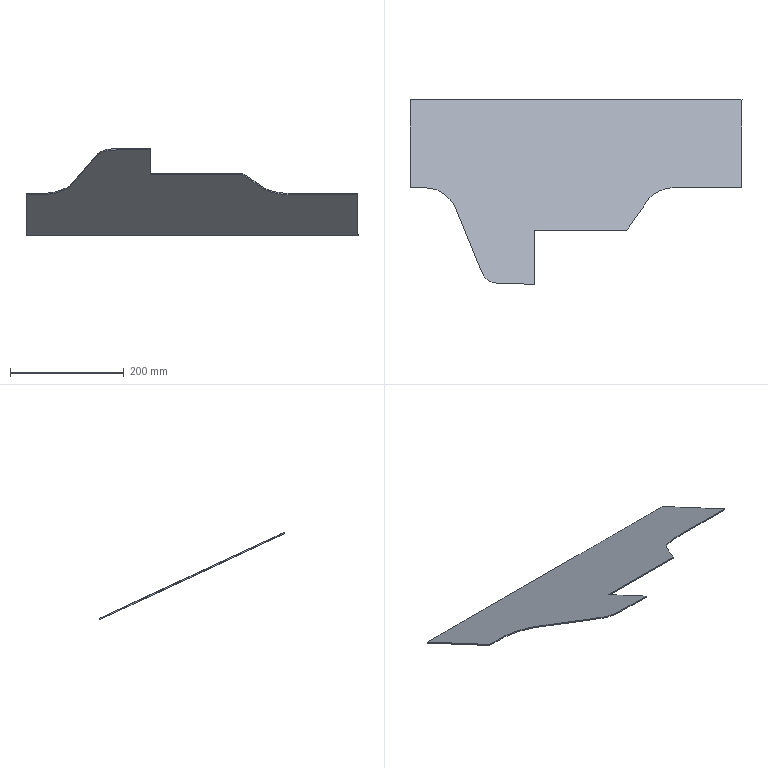Part | NX | features solid 2 | 1 solid | 9 faces | box 585 x 325.491 x 153.986 mm | volume 277101 mm3 | plane 7 | spline 2
STEP:
#1=CARTESIAN_POINT('',(-15.,64.511,-80.89));
#2=VERTEX_POINT('',#1);
#3=CARTESIAN_POINT('',(-235.,234.941,-160.363));
#4=VERTEX_POINT('',#3);
#5=CARTESIAN_POINT('',(-15.,64.511,-80.89));
#6=CARTESIAN_POINT('',(-18.445,64.501,-80.885));
#7=CARTESIAN_POINT('',(-25.333,64.55,-80.908));
#8=CARTESIAN_POINT('',(-35.665,64.778,-81.014));
#9=CARTESIAN_POINT('',(-45.997,65.047,-81.14));
#10=CARTESIAN_POINT('',(-56.325,65.488,-81.346));
#11=CARTESIAN_POINT('',(-66.665,65.754,-81.47));
#12=CARTESIAN_POINT('',(-76.969,65.677,-81.434));
#13=CARTESIAN_POINT('',(-87.409,66.786,-81.951));
#14=CARTESIAN_POINT('',(-97.044,70.795,-83.82));
#15=CARTESIAN_POINT('',(-104.46,77.651,-87.017));
#16=CARTESIAN_POINT('',(-109.205,86.072,-90.944));
#17=CARTESIAN_POINT('',(-112.555,95.072,-95.141));
#18=CARTESIAN_POINT('',(-115.959,104.022,-99.314));
#19=CARTESIAN_POINT('',(-119.506,112.932,-103.469));
#20=CARTESIAN_POINT('',(-123.05,121.84,-107.623));
#21=CARTESIAN_POINT('',(-126.716,130.709,-111.759));
#22=CARTESIAN_POINT('',(-131.727,142.492,-117.253));
#23=CARTESIAN_POINT('',(-138.057,157.199,-124.111));
#24=CARTESIAN_POINT('',(-144.248,171.953,-130.991));
#25=CARTESIAN_POINT('',(-148.845,183.875,-136.55));
#26=CARTESIAN_POINT('',(-152.222,192.846,-140.733));
#27=CARTESIAN_POINT('',(-155.816,201.72,-144.872));
#28=CARTESIAN_POINT('',(-160.656,210.149,-148.802));
#29=CARTESIAN_POINT('',(-167.167,217.758,-152.35));
#30=CARTESIAN_POINT('',(-174.848,224.259,-155.382));
#31=CARTESIAN_POINT('',(-183.675,229.58,-157.863));
#32=CARTESIAN_POINT('',(-191.706,232.657,-159.298));
#33=CARTESIAN_POINT('',(-198.651,234.08,-159.962));
#34=CARTESIAN_POINT('',(-205.542,234.889,-160.338));
#35=CARTESIAN_POINT('',(-214.207,235.059,-160.418));
#36=CARTESIAN_POINT('',(-224.604,234.94,-160.362));
#37=CARTESIAN_POINT('',(-231.535,234.942,-160.363));
#38=CARTESIAN_POINT('',(-235.,234.941,-160.363));
#39=B_SPLINE_CURVE_WITH_KNOTS('',3,(#5,#6,#7,#8,#9,#10,#11,#12,#13,#14,#15,#16,#17,#18,#19,#20,#21,#22,#23,#24,#25,#26,#27,#28,#29,#30,#31,#32,#33,#34,#35,#36,#37,#38),.UNSPECIFIED.,.F.,.F.,(4,1,1,1,1,1,1,1,1,1,1,1,1,1,1,1,1,1,1,1,1,1,1,1,1,1,1,1,1,1,1,4),(0.4481,0.4583,0.4685,0.4788,0.489,0.4992,0.5095,0.5197,0.5299,0.5402,0.5504,0.5606,0.5709,0.5811,0.5914,0.6016,0.6118,0.6323,0.6528,0.663,0.6732,0.6835,0.6937,0.7039,0.7142,0.7244,0.7346,0.7398,0.7449,0.7551,0.7654,0.7756),.UNSPECIFIED.);
#40=EDGE_CURVE('',#2,#4,#39,.T.);
#41=ORIENTED_EDGE('',*,*,#40,.F.);
#42=CARTESIAN_POINT('',(-15.,160.,-125.417));
#43=VERTEX_POINT('',#42);
#44=CARTESIAN_POINT('',(-15.,512.511,-289.796));
#45=DIRECTION('',(0.,0.9063,-0.4226));
#46=VECTOR('',#45,1000.);
#47=LINE('',#44,#46);
#48=EDGE_CURVE('',#2,#43,#47,.T.);
#49=ORIENTED_EDGE('',*,*,#48,.T.);
#50=CARTESIAN_POINT('',(147.311,160.,-125.417));
#51=VERTEX_POINT('',#50);
#52=CARTESIAN_POINT('',(45.,160.,-125.417));
#53=DIRECTION('',(1.,0.,0.));
#54=VECTOR('',#53,1000.);
#55=LINE('',#52,#54);
#56=EDGE_CURVE('',#43,#51,#55,.T.);
#57=ORIENTED_EDGE('',*,*,#56,.T.);
#58=CARTESIAN_POINT('',(350.,234.942,-160.363));
#59=VERTEX_POINT('',#58);
#60=CARTESIAN_POINT('',(350.,234.942,-160.363));
#61=CARTESIAN_POINT('',(339.975,234.936,-160.361));
#62=CARTESIAN_POINT('',(324.937,234.935,-160.36));
#63=CARTESIAN_POINT('',(304.886,234.96,-160.372));
#64=CARTESIAN_POINT('',(289.848,234.985,-160.383));
#65=CARTESIAN_POINT('',(274.811,234.996,-160.388));
#66=CARTESIAN_POINT('',(259.772,234.948,-160.366));
#67=CARTESIAN_POINT('',(247.244,234.881,-160.335));
#68=CARTESIAN_POINT('',(237.205,235.037,-160.408));
#69=CARTESIAN_POINT('',(229.686,235.041,-160.41));
#70=CARTESIAN_POINT('',(222.219,234.482,-160.149));
#71=CARTESIAN_POINT('',(214.845,233.031,-159.472));
#72=CARTESIAN_POINT('',(207.533,230.61,-158.343));
#73=CARTESIAN_POINT('',(200.799,227.39,-156.842));
#74=CARTESIAN_POINT('',(194.539,223.399,-154.981));
#75=CARTESIAN_POINT('',(188.818,218.647,-152.765));
#76=CARTESIAN_POINT('',(183.898,213.367,-150.303));
#77=CARTESIAN_POINT('',(179.607,207.587,-147.608));
#78=CARTESIAN_POINT('',(175.69,201.565,-144.799));
#79=CARTESIAN_POINT('',(170.518,193.522,-141.049));
#80=CARTESIAN_POINT('',(163.791,183.604,-136.424));
#81=CARTESIAN_POINT('',(155.579,171.787,-130.914));
#82=CARTESIAN_POINT('',(150.08,163.921,-127.246));
#83=CARTESIAN_POINT('',(147.311,160.,-125.417));
#84=B_SPLINE_CURVE_WITH_KNOTS('',3,(#60,#61,#62,#63,#64,#65,#66,#67,#68,#69,#70,#71,#72,#73,#74,#75,#76,#77,#78,#79,#80,#81,#82,#83),.UNSPECIFIED.,.F.,.F.,(4,1,1,1,1,1,1,1,1,1,1,1,1,1,1,1,1,1,1,1,1,4),(0.,0.03008,0.04511,0.06015,0.07519,0.09023,0.1053,0.1128,0.1203,0.1278,0.1353,0.1429,0.1504,0.1579,0.1654,0.1729,0.1805,0.188,0.1955,0.2105,0.2256,0.2406),.UNSPECIFIED.);
#85=EDGE_CURVE('',#59,#51,#84,.T.);
#86=ORIENTED_EDGE('',*,*,#85,.F.);
#87=CARTESIAN_POINT('',(350.,390.,-232.668));
#88=VERTEX_POINT('',#87);
#89=CARTESIAN_POINT('',(350.,287.2,-184.732));
#90=DIRECTION('',(0.,-0.9063,0.4226));
#91=VECTOR('',#90,1000.);
#92=LINE('',#89,#91);
#93=EDGE_CURVE('',#88,#59,#92,.T.);
#94=ORIENTED_EDGE('',*,*,#93,.F.);
#95=CARTESIAN_POINT('',(-235.,390.,-232.668));
#96=VERTEX_POINT('',#95);
#97=CARTESIAN_POINT('',(45.,390.,-232.668));
#98=DIRECTION('',(-1.,0.,0.));
#99=VECTOR('',#98,1000.);
#100=LINE('',#97,#99);
#101=EDGE_CURVE('',#88,#96,#100,.T.);
#102=ORIENTED_EDGE('',*,*,#101,.T.);
#103=CARTESIAN_POINT('',(-235.,512.511,-289.796));
#104=DIRECTION('',(0.,0.9063,-0.4226));
#105=VECTOR('',#104,1000.);
#106=LINE('',#103,#105);
#107=EDGE_CURVE('',#96,#4,#106,.F.);
#108=ORIENTED_EDGE('',*,*,#107,.T.);
#109=EDGE_LOOP('',(#41,#49,#57,#86,#94,#102,#108));
#110=FACE_BOUND('',#109,.T.);
#111=CARTESIAN_POINT('',(45.,512.511,-289.796));
#112=DIRECTION('',(0.,0.4226,0.9063));
#113=DIRECTION('',(1.,0.,0.));
#114=AXIS2_PLACEMENT_3D('',#111,#112,#113);
#115=PLANE('',#114);
#116=ADVANCED_FACE('',(#110),#115,.T.);
#117=CARTESIAN_POINT('',(-15.,64.511,-83.097));
#118=VERTEX_POINT('',#117);
#119=CARTESIAN_POINT('',(-15.,160.,-127.624));
#120=VERTEX_POINT('',#119);
#121=CARTESIAN_POINT('',(-15.,175.818,-135.));
#122=DIRECTION('',(0.,0.9063,-0.4226));
#123=VECTOR('',#122,1000.);
#124=LINE('',#121,#123);
#125=EDGE_CURVE('',#118,#120,#124,.T.);
#126=ORIENTED_EDGE('',*,*,#125,.F.);
#127=CARTESIAN_POINT('',(-235.,234.941,-162.57));
#128=VERTEX_POINT('',#127);
#129=CARTESIAN_POINT('',(-15.,64.511,-83.097));
#130=CARTESIAN_POINT('',(-18.445,64.501,-83.092));
#131=CARTESIAN_POINT('',(-25.333,64.55,-83.115));
#132=CARTESIAN_POINT('',(-35.665,64.778,-83.221));
#133=CARTESIAN_POINT('',(-45.997,65.047,-83.347));
#134=CARTESIAN_POINT('',(-56.325,65.488,-83.552));
#135=CARTESIAN_POINT('',(-66.665,65.754,-83.676));
#136=CARTESIAN_POINT('',(-76.969,65.677,-83.641));
#137=CARTESIAN_POINT('',(-87.409,66.786,-84.158));
#138=CARTESIAN_POINT('',(-97.044,70.795,-86.027));
#139=CARTESIAN_POINT('',(-104.46,77.651,-89.224));
#140=CARTESIAN_POINT('',(-109.205,86.072,-93.151));
#141=CARTESIAN_POINT('',(-112.555,95.072,-97.348));
#142=CARTESIAN_POINT('',(-115.959,104.022,-101.521));
#143=CARTESIAN_POINT('',(-119.506,112.932,-105.676));
#144=CARTESIAN_POINT('',(-123.05,121.84,-109.83));
#145=CARTESIAN_POINT('',(-126.716,130.709,-113.965));
#146=CARTESIAN_POINT('',(-131.727,142.492,-119.46));
#147=CARTESIAN_POINT('',(-138.057,157.199,-126.318));
#148=CARTESIAN_POINT('',(-144.248,171.953,-133.198));
#149=CARTESIAN_POINT('',(-148.845,183.875,-138.757));
#150=CARTESIAN_POINT('',(-152.222,192.846,-142.94));
#151=CARTESIAN_POINT('',(-155.816,201.72,-147.078));
#152=CARTESIAN_POINT('',(-160.656,210.149,-151.009));
#153=CARTESIAN_POINT('',(-167.167,217.758,-154.557));
#154=CARTESIAN_POINT('',(-174.848,224.259,-157.588));
#155=CARTESIAN_POINT('',(-183.675,229.58,-160.07));
#156=CARTESIAN_POINT('',(-191.706,232.657,-161.504));
#157=CARTESIAN_POINT('',(-198.651,234.08,-162.168));
#158=CARTESIAN_POINT('',(-205.542,234.889,-162.545));
#159=CARTESIAN_POINT('',(-214.207,235.059,-162.624));
#160=CARTESIAN_POINT('',(-224.604,234.94,-162.569));
#161=CARTESIAN_POINT('',(-231.535,234.942,-162.57));
#162=CARTESIAN_POINT('',(-235.,234.941,-162.57));
#163=B_SPLINE_CURVE_WITH_KNOTS('',3,(#129,#130,#131,#132,#133,#134,#135,#136,#137,#138,#139,#140,#141,#142,#143,#144,#145,#146,#147,#148,#149,#150,#151,#152,#153,#154,#155,#156,#157,#158,#159,#160,#161,#162),.UNSPECIFIED.,.F.,.F.,(4,1,1,1,1,1,1,1,1,1,1,1,1,1,1,1,1,1,1,1,1,1,1,1,1,1,1,1,1,1,1,4),(0.4481,0.4583,0.4685,0.4788,0.489,0.4992,0.5095,0.5197,0.5299,0.5402,0.5504,0.5606,0.5709,0.5811,0.5914,0.6016,0.6118,0.6323,0.6528,0.663,0.6732,0.6835,0.6937,0.7039,0.7142,0.7244,0.7346,0.7398,0.7449,0.7551,0.7654,0.7756),.UNSPECIFIED.);
#164=EDGE_CURVE('',#118,#128,#163,.T.);
#165=ORIENTED_EDGE('',*,*,#164,.T.);
#166=CARTESIAN_POINT('',(-235.,390.,-234.875));
#167=VERTEX_POINT('',#166);
#168=CARTESIAN_POINT('',(-235.,175.818,-135.));
#169=DIRECTION('',(0.,0.9063,-0.4226));
#170=VECTOR('',#169,1000.);
#171=LINE('',#168,#170);
#172=EDGE_CURVE('',#167,#128,#171,.F.);
#173=ORIENTED_EDGE('',*,*,#172,.F.);
#174=CARTESIAN_POINT('',(350.,390.,-234.875));
#175=VERTEX_POINT('',#174);
#176=CARTESIAN_POINT('',(-950.,390.,-234.875));
#177=DIRECTION('',(-1.,0.,0.));
#178=VECTOR('',#177,1000.);
#179=LINE('',#176,#178);
#180=EDGE_CURVE('',#175,#167,#179,.T.);
#181=ORIENTED_EDGE('',*,*,#180,.F.);
#182=CARTESIAN_POINT('',(350.,234.942,-162.57));
#183=VERTEX_POINT('',#182);
#184=CARTESIAN_POINT('',(350.,286.355,-186.544));
#185=DIRECTION('',(0.,-0.9063,0.4226));
#186=VECTOR('',#185,1000.);
#187=LINE('',#184,#186);
#188=EDGE_CURVE('',#175,#183,#187,.T.);
#189=ORIENTED_EDGE('',*,*,#188,.T.);
#190=CARTESIAN_POINT('',(147.311,160.,-127.624));
#191=VERTEX_POINT('',#190);
#192=CARTESIAN_POINT('',(350.,234.942,-162.57));
#193=CARTESIAN_POINT('',(339.975,234.936,-162.567));
#194=CARTESIAN_POINT('',(324.937,234.935,-162.567));
#195=CARTESIAN_POINT('',(304.886,234.96,-162.579));
#196=CARTESIAN_POINT('',(289.848,234.985,-162.59));
#197=CARTESIAN_POINT('',(274.811,234.996,-162.595));
#198=CARTESIAN_POINT('',(259.772,234.948,-162.573));
#199=CARTESIAN_POINT('',(247.244,234.881,-162.542));
#200=CARTESIAN_POINT('',(237.205,235.037,-162.614));
#201=CARTESIAN_POINT('',(229.686,235.041,-162.616));
#202=CARTESIAN_POINT('',(222.219,234.482,-162.356));
#203=CARTESIAN_POINT('',(214.845,233.031,-161.679));
#204=CARTESIAN_POINT('',(207.533,230.61,-160.55));
#205=CARTESIAN_POINT('',(200.799,227.39,-159.048));
#206=CARTESIAN_POINT('',(194.539,223.399,-157.187));
#207=CARTESIAN_POINT('',(188.818,218.647,-154.972));
#208=CARTESIAN_POINT('',(183.898,213.367,-152.509));
#209=CARTESIAN_POINT('',(179.607,207.587,-149.814));
#210=CARTESIAN_POINT('',(175.69,201.565,-147.006));
#211=CARTESIAN_POINT('',(170.518,193.522,-143.255));
#212=CARTESIAN_POINT('',(163.791,183.604,-138.631));
#213=CARTESIAN_POINT('',(155.579,171.787,-133.12));
#214=CARTESIAN_POINT('',(150.08,163.921,-129.453));
#215=CARTESIAN_POINT('',(147.311,160.,-127.624));
#216=B_SPLINE_CURVE_WITH_KNOTS('',3,(#192,#193,#194,#195,#196,#197,#198,#199,#200,#201,#202,#203,#204,#205,#206,#207,#208,#209,#210,#211,#212,#213,#214,#215),.UNSPECIFIED.,.F.,.F.,(4,1,1,1,1,1,1,1,1,1,1,1,1,1,1,1,1,1,1,1,1,4),(0.,0.03008,0.04511,0.06015,0.07519,0.09023,0.1053,0.1128,0.1203,0.1278,0.1353,0.1429,0.1504,0.1579,0.1654,0.1729,0.1805,0.188,0.1955,0.2105,0.2256,0.2406),.UNSPECIFIED.);
#217=EDGE_CURVE('',#183,#191,#216,.T.);
#218=ORIENTED_EDGE('',*,*,#217,.T.);
#219=CARTESIAN_POINT('',(-950.,160.,-127.624));
#220=DIRECTION('',(1.,0.,0.));
#221=VECTOR('',#220,1000.);
#222=LINE('',#219,#221);
#223=EDGE_CURVE('',#120,#191,#222,.T.);
#224=ORIENTED_EDGE('',*,*,#223,.F.);
#225=EDGE_LOOP('',(#126,#165,#173,#181,#189,#218,#224));
#226=FACE_BOUND('',#225,.T.);
#227=CARTESIAN_POINT('',(-950.,175.818,-135.));
#228=DIRECTION('',(0.,0.4226,0.9063));
#229=DIRECTION('',(0.,-0.9063,0.4226));
#230=AXIS2_PLACEMENT_3D('',#227,#228,#229);
#231=PLANE('',#230);
#232=ADVANCED_FACE('',(#226),#231,.F.);
#233=ORIENTED_EDGE('',*,*,#101,.F.);
#234=CARTESIAN_POINT('',(350.,390.,-145.));
#235=DIRECTION('',(0.,0.,-1.));
#236=VECTOR('',#235,1000.);
#237=LINE('',#234,#236);
#238=EDGE_CURVE('',#88,#175,#237,.T.);
#239=ORIENTED_EDGE('',*,*,#238,.T.);
#240=ORIENTED_EDGE('',*,*,#180,.T.);
#241=CARTESIAN_POINT('',(-235.,390.,-327.54));
#242=DIRECTION('',(0.,0.,1.));
#243=VECTOR('',#242,1000.);
#244=LINE('',#241,#243);
#245=EDGE_CURVE('',#96,#167,#244,.F.);
#246=ORIENTED_EDGE('',*,*,#245,.F.);
#247=EDGE_LOOP('',(#233,#239,#240,#246));
#248=FACE_BOUND('',#247,.T.);
#249=CARTESIAN_POINT('',(455.,390.,-145.));
#250=DIRECTION('',(0.,1.,0.));
#251=DIRECTION('',(0.,0.,-1.));
#252=AXIS2_PLACEMENT_3D('',#249,#250,#251);
#253=PLANE('',#252);
#254=ADVANCED_FACE('',(#248),#253,.T.);
#255=CARTESIAN_POINT('',(-15.,64.511,-121.239));
#256=DIRECTION('',(0.,0.,-1.));
#257=VECTOR('',#256,1000.);
#258=LINE('',#255,#257);
#259=EDGE_CURVE('',#2,#118,#258,.T.);
#260=ORIENTED_EDGE('',*,*,#259,.F.);
#261=ORIENTED_EDGE('',*,*,#40,.T.);
#262=CARTESIAN_POINT('',(-235.,234.941,-161.472));
#263=DIRECTION('',(0.,0.,-1.));
#264=VECTOR('',#263,1000.);
#265=LINE('',#262,#264);
#266=EDGE_CURVE('',#4,#128,#265,.T.);
#267=ORIENTED_EDGE('',*,*,#266,.T.);
#268=ORIENTED_EDGE('',*,*,#164,.F.);
#269=EDGE_LOOP('',(#260,#261,#267,#268));
#270=FACE_BOUND('',#269,.T.);
#271=CARTESIAN_POINT('',(-235.,234.941,-79.524));
#272=CARTESIAN_POINT('',(-235.,234.941,-163.701));
#273=CARTESIAN_POINT('',(-231.678,234.942,-79.524));
#274=CARTESIAN_POINT('',(-231.678,234.942,-163.701));
#275=CARTESIAN_POINT('',(-225.038,234.941,-79.524));
#276=CARTESIAN_POINT('',(-225.038,234.941,-163.701));
#277=CARTESIAN_POINT('',(-215.058,235.044,-79.524));
#278=CARTESIAN_POINT('',(-215.058,235.044,-163.701));
#279=CARTESIAN_POINT('',(-205.091,234.915,-79.524));
#280=CARTESIAN_POINT('',(-205.091,234.915,-163.701));
#281=CARTESIAN_POINT('',(-195.172,233.672,-79.524));
#282=CARTESIAN_POINT('',(-195.172,233.672,-163.701));
#283=CARTESIAN_POINT('',(-185.67,230.508,-79.524));
#284=CARTESIAN_POINT('',(-185.67,230.508,-163.701));
#285=CARTESIAN_POINT('',(-176.916,225.67,-79.524));
#286=CARTESIAN_POINT('',(-176.916,225.67,-163.701));
#287=CARTESIAN_POINT('',(-169.03,219.526,-79.524));
#288=CARTESIAN_POINT('',(-169.03,219.526,-163.701));
#289=CARTESIAN_POINT('',(-162.191,212.204,-79.524));
#290=CARTESIAN_POINT('',(-162.191,212.204,-163.701));
#291=CARTESIAN_POINT('',(-156.804,203.807,-79.524));
#292=CARTESIAN_POINT('',(-156.804,203.807,-163.701));
#293=CARTESIAN_POINT('',(-152.887,194.628,-79.524));
#294=CARTESIAN_POINT('',(-152.887,194.628,-163.701));
#295=CARTESIAN_POINT('',(-149.376,185.265,-79.524));
#296=CARTESIAN_POINT('',(-149.376,185.265,-163.701));
#297=CARTESIAN_POINT('',(-144.62,172.874,-79.524));
#298=CARTESIAN_POINT('',(-144.62,172.874,-163.701));
#299=CARTESIAN_POINT('',(-138.21,157.543,-79.524));
#300=CARTESIAN_POINT('',(-138.21,157.543,-163.701));
#301=CARTESIAN_POINT('',(-131.638,142.287,-79.524));
#302=CARTESIAN_POINT('',(-131.638,142.287,-163.701));
#303=CARTESIAN_POINT('',(-126.44,130.056,-79.524));
#304=CARTESIAN_POINT('',(-126.44,130.056,-163.701));
#305=CARTESIAN_POINT('',(-122.644,120.84,-79.524));
#306=CARTESIAN_POINT('',(-122.644,120.84,-163.701));
#307=CARTESIAN_POINT('',(-118.971,111.575,-79.524));
#308=CARTESIAN_POINT('',(-118.971,111.575,-163.701));
#309=CARTESIAN_POINT('',(-115.278,102.315,-79.524));
#310=CARTESIAN_POINT('',(-115.278,102.315,-163.701));
#311=CARTESIAN_POINT('',(-111.803,92.98,-79.524));
#312=CARTESIAN_POINT('',(-111.803,92.98,-163.701));
#313=CARTESIAN_POINT('',(-108.16,83.678,-79.524));
#314=CARTESIAN_POINT('',(-108.16,83.678,-163.701));
#315=CARTESIAN_POINT('',(-102.524,75.335,-79.524));
#316=CARTESIAN_POINT('',(-102.524,75.335,-163.701));
#317=CARTESIAN_POINT('',(-94.368,69.314,-79.524));
#318=CARTESIAN_POINT('',(-94.368,69.314,-163.701));
#319=CARTESIAN_POINT('',(-84.772,66.318,-79.524));
#320=CARTESIAN_POINT('',(-84.772,66.318,-163.701));
#321=CARTESIAN_POINT('',(-74.812,65.672,-79.524));
#322=CARTESIAN_POINT('',(-74.812,65.672,-163.701));
#323=CARTESIAN_POINT('',(-64.802,65.749,-79.524));
#324=CARTESIAN_POINT('',(-64.802,65.749,-163.701));
#325=CARTESIAN_POINT('',(-54.86,65.409,-79.524));
#326=CARTESIAN_POINT('',(-54.86,65.409,-163.701));
#327=CARTESIAN_POINT('',(-44.895,65.018,-79.524));
#328=CARTESIAN_POINT('',(-44.895,65.018,-163.701));
#329=CARTESIAN_POINT('',(-31.612,64.671,-79.524));
#330=CARTESIAN_POINT('',(-31.612,64.671,-163.701));
#331=CARTESIAN_POINT('',(-21.645,64.492,-79.524));
#332=CARTESIAN_POINT('',(-21.645,64.492,-163.701));
#333=CARTESIAN_POINT('',(-15.,64.511,-79.524));
#334=CARTESIAN_POINT('',(-15.,64.511,-163.701));
#335=B_SPLINE_SURFACE_WITH_KNOTS('',3,1,((#271,#272),(#273,#274),(#275,#276),(#277,#278),(#279,#280),(#281,#282),(#283,#284),(#285,#286),(#287,#288),(#289,#290),(#291,#292),(#293,#294),(#295,#296),(#297,#298),(#299,#300),(#301,#302),(#303,#304),(#305,#306),(#307,#308),(#309,#310),(#311,#312),(#313,#314),(#315,#316),(#317,#318),(#319,#320),(#321,#322),(#323,#324),(#325,#326),(#327,#328),(#329,#330),(#331,#332),(#333,#334)),.SURF_OF_LINEAR_EXTRUSION.,.F.,.F.,.F.,(4,1,1,1,1,1,1,1,1,1,1,1,1,1,1,1,1,1,1,1,1,1,1,1,1,1,1,1,1,4),(2,2),(0.6464,0.6486,0.6508,0.653,0.6552,0.6574,0.6596,0.6618,0.6639,0.6661,0.6683,0.6705,0.6727,0.6771,0.6815,0.6837,0.6859,0.6881,0.6903,0.6924,0.6946,0.6968,0.699,0.7012,0.7034,0.7056,0.7078,0.71,0.7122,0.7166),(0.,1.),.UNSPECIFIED.);
#336=ADVANCED_FACE('',(#270),#335,.F.);
#337=ORIENTED_EDGE('',*,*,#266,.F.);
#338=ORIENTED_EDGE('',*,*,#107,.F.);
#339=ORIENTED_EDGE('',*,*,#245,.T.);
#340=ORIENTED_EDGE('',*,*,#172,.T.);
#341=EDGE_LOOP('',(#337,#338,#339,#340));
#342=FACE_BOUND('',#341,.T.);
#343=CARTESIAN_POINT('',(-235.,154.934,-327.54));
#344=DIRECTION('',(1.,-0.000000001,0.));
#345=DIRECTION('',(0.000000001,1.,0.));
#346=AXIS2_PLACEMENT_3D('',#343,#344,#345);
#347=PLANE('',#346);
#348=ADVANCED_FACE('',(#342),#347,.F.);
#349=CARTESIAN_POINT('',(-15.,160.,-415.));
#350=DIRECTION('',(0.,0.,-1.));
#351=VECTOR('',#350,1000.);
#352=LINE('',#349,#351);
#353=EDGE_CURVE('',#43,#120,#352,.T.);
#354=ORIENTED_EDGE('',*,*,#353,.F.);
#355=ORIENTED_EDGE('',*,*,#48,.F.);
#356=ORIENTED_EDGE('',*,*,#259,.T.);
#357=ORIENTED_EDGE('',*,*,#125,.T.);
#358=EDGE_LOOP('',(#354,#355,#356,#357));
#359=FACE_BOUND('',#358,.T.);
#360=CARTESIAN_POINT('',(-15.,160.,-415.));
#361=DIRECTION('',(1.,0.,0.));
#362=DIRECTION('',(0.,0.,-1.));
#363=AXIS2_PLACEMENT_3D('',#360,#361,#362);
#364=PLANE('',#363);
#365=ADVANCED_FACE('',(#359),#364,.T.);
#366=CARTESIAN_POINT('',(147.311,160.,-121.582));
#367=DIRECTION('',(0.,0.,-1.));
#368=VECTOR('',#367,1000.);
#369=LINE('',#366,#368);
#370=EDGE_CURVE('',#191,#51,#369,.F.);
#371=ORIENTED_EDGE('',*,*,#370,.F.);
#372=ORIENTED_EDGE('',*,*,#217,.F.);
#373=CARTESIAN_POINT('',(350.,234.942,600.));
#374=DIRECTION('',(0.,0.,-1.));
#375=VECTOR('',#374,1000.);
#376=LINE('',#373,#375);
#377=EDGE_CURVE('',#183,#59,#376,.F.);
#378=ORIENTED_EDGE('',*,*,#377,.T.);
#379=ORIENTED_EDGE('',*,*,#85,.T.);
#380=EDGE_LOOP('',(#371,#372,#378,#379));
#381=FACE_BOUND('',#380,.T.);
#382=CARTESIAN_POINT('',(147.311,160.,-125.192));
#383=CARTESIAN_POINT('',(147.311,160.,-163.23));
#384=CARTESIAN_POINT('',(150.161,164.036,-125.192));
#385=CARTESIAN_POINT('',(150.161,164.036,-163.23));
#386=CARTESIAN_POINT('',(155.821,172.137,-125.192));
#387=CARTESIAN_POINT('',(155.821,172.137,-163.23));
#388=CARTESIAN_POINT('',(164.284,184.309,-125.192));
#389=CARTESIAN_POINT('',(164.284,184.309,-163.23));
#390=CARTESIAN_POINT('',(171.195,194.546,-125.192));
#391=CARTESIAN_POINT('',(171.195,194.546,-163.23));
#392=CARTESIAN_POINT('',(176.52,202.872,-125.192));
#393=CARTESIAN_POINT('',(176.52,202.872,-163.23));
#394=CARTESIAN_POINT('',(180.617,209.051,-125.192));
#395=CARTESIAN_POINT('',(180.617,209.051,-163.23));
#396=CARTESIAN_POINT('',(185.186,214.9,-125.192));
#397=CARTESIAN_POINT('',(185.186,214.9,-163.23));
#398=CARTESIAN_POINT('',(192.209,221.88,-125.192));
#399=CARTESIAN_POINT('',(192.209,221.88,-163.23));
#400=CARTESIAN_POINT('',(202.539,228.833,-125.192));
#401=CARTESIAN_POINT('',(202.539,228.833,-163.23));
#402=CARTESIAN_POINT('',(214.238,233.067,-125.192));
#403=CARTESIAN_POINT('',(214.238,233.067,-163.23));
#404=CARTESIAN_POINT('',(224.006,234.693,-125.192));
#405=CARTESIAN_POINT('',(224.006,234.693,-163.23));
#406=CARTESIAN_POINT('',(231.403,235.07,-125.192));
#407=CARTESIAN_POINT('',(231.403,235.07,-163.23));
#408=CARTESIAN_POINT('',(238.823,235.006,-125.192));
#409=CARTESIAN_POINT('',(238.823,235.006,-163.23));
#410=CARTESIAN_POINT('',(248.712,234.881,-125.192));
#411=CARTESIAN_POINT('',(248.712,234.881,-163.23));
#412=CARTESIAN_POINT('',(261.058,234.957,-125.192));
#413=CARTESIAN_POINT('',(261.058,234.957,-163.23));
#414=CARTESIAN_POINT('',(275.883,234.996,-125.192));
#415=CARTESIAN_POINT('',(275.883,234.996,-163.23));
#416=CARTESIAN_POINT('',(290.707,234.984,-125.192));
#417=CARTESIAN_POINT('',(290.707,234.984,-163.23));
#418=CARTESIAN_POINT('',(305.53,234.959,-125.192));
#419=CARTESIAN_POINT('',(305.53,234.959,-163.23));
#420=CARTESIAN_POINT('',(325.294,234.935,-125.192));
#421=CARTESIAN_POINT('',(325.294,234.935,-163.23));
#422=CARTESIAN_POINT('',(340.118,234.936,-125.192));
#423=CARTESIAN_POINT('',(340.118,234.936,-163.23));
#424=CARTESIAN_POINT('',(350.,234.942,-125.192));
#425=CARTESIAN_POINT('',(350.,234.942,-163.23));
#426=B_SPLINE_SURFACE_WITH_KNOTS('',3,1,((#382,#383),(#384,#385),(#386,#387),(#388,#389),(#390,#391),(#392,#393),(#394,#395),(#396,#397),(#398,#399),(#400,#401),(#402,#403),(#404,#405),(#406,#407),(#408,#409),(#410,#411),(#412,#413),(#414,#415),(#416,#417),(#418,#419),(#420,#421),(#422,#423),(#424,#425)),.SURF_OF_LINEAR_EXTRUSION.,.F.,.F.,.F.,(4,1,1,1,1,1,1,1,1,1,1,1,1,1,1,1,1,1,1,4),(2,2),(0.7617,0.7649,0.7682,0.7715,0.7731,0.7747,0.7763,0.778,0.7812,0.7845,0.7861,0.7878,0.7894,0.791,0.7943,0.7975,0.8008,0.8041,0.8073,0.8138),(0.,1.),.UNSPECIFIED.);
#427=ADVANCED_FACE('',(#381),#426,.F.);
#428=ORIENTED_EDGE('',*,*,#377,.F.);
#429=ORIENTED_EDGE('',*,*,#188,.F.);
#430=ORIENTED_EDGE('',*,*,#238,.F.);
#431=ORIENTED_EDGE('',*,*,#93,.T.);
#432=EDGE_LOOP('',(#428,#429,#430,#431));
#433=FACE_BOUND('',#432,.T.);
#434=CARTESIAN_POINT('',(350.,229.934,-307.54));
#435=DIRECTION('',(1.,0.,0.));
#436=DIRECTION('',(0.,1.,0.));
#437=AXIS2_PLACEMENT_3D('',#434,#435,#436);
#438=PLANE('',#437);
#439=ADVANCED_FACE('',(#433),#438,.T.);
#440=ORIENTED_EDGE('',*,*,#223,.T.);
#441=ORIENTED_EDGE('',*,*,#370,.T.);
#442=ORIENTED_EDGE('',*,*,#56,.F.);
#443=ORIENTED_EDGE('',*,*,#353,.T.);
#444=EDGE_LOOP('',(#440,#441,#442,#443));
#445=FACE_BOUND('',#444,.T.);
#446=CARTESIAN_POINT('',(5.,160.,-125.));
#447=DIRECTION('',(0.,-1.,0.));
#448=DIRECTION('',(1.,0.,0.));
#449=AXIS2_PLACEMENT_3D('',#446,#447,#448);
#450=PLANE('',#449);
#451=ADVANCED_FACE('',(#445),#450,.T.);
#452=CLOSED_SHELL('',(#116,#232,#254,#336,#348,#365,#427,#439,#451));
#453=MANIFOLD_SOLID_BREP('',#452);
#454=(LENGTH_UNIT()NAMED_UNIT(*)SI_UNIT(.MILLI.,.METRE.));
#455=UNCERTAINTY_MEASURE_WITH_UNIT(LENGTH_MEASURE(0.0508),#454,'','');
#456=(NAMED_UNIT(*)PLANE_ANGLE_UNIT()SI_UNIT($,.RADIAN.));
#457=(NAMED_UNIT(*)SI_UNIT($,.STERADIAN.)SOLID_ANGLE_UNIT());
#458=(GEOMETRIC_REPRESENTATION_CONTEXT(3)GLOBAL_UNCERTAINTY_ASSIGNED_CONTEXT((#455))GLOBAL_UNIT_ASSIGNED_CONTEXT((#454,#456,#457))REPRESENTATION_CONTEXT('',''));
#459=ADVANCED_BREP_SHAPE_REPRESENTATION('',(#453),#458);